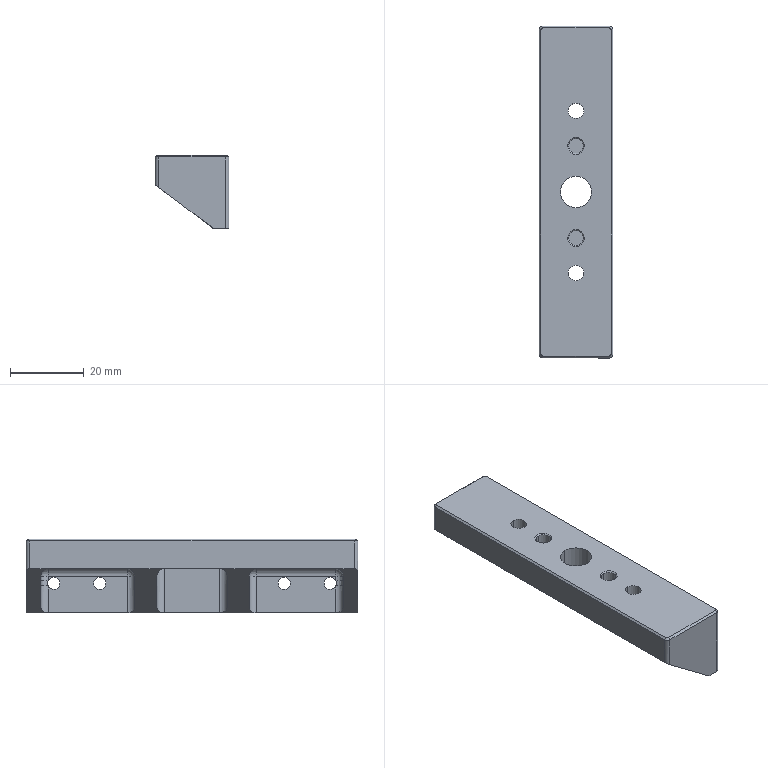NC program | NX | posted with a generic post | part box 20 x 90 x 20 mm
Whole program:
N10 G17 G21 G94 G90
(DRILLING_COPY , TOOL : D6A45)
N12 T01 M6
N14 G54
N16 G17 G0 G90 X-37.5 Y-2. B0. C0. S5000 M3
N18 G43 Z30. H1
N20 G94 G81 G98 Z-1. F350. R3.
N22 X-25.
N24 X-12.5
N26 X12.5
N28 X25.
N30 X37.5
N32 G80
N34 G0 X37.5 Y-2. Z30.
N36 M5
(DRILLING_COPY_1 , TOOL : 3.3ZT)
N38 T03 M6
N40 G54
N42 G17 G0 G90 X-37.5 Y-2. B0. C0. S2000 M3
N44 G43 Z30. H3
N46 G94 G83 G98 Z-6.491 F200. Q2. R3.
N48 X-25.
N50 X25.
N52 X37.5
N54 G80
N56 G0 X37.5 Y-2. Z30.
N58 M5
(DRILLING_COPY_COPY_1_COPY_COPY , TOOL : 3.8ZT)
N60 T18 M6
N62 G54
N64 G17 G0 G90 X12.5 Y-2. B0. C0. S2000 M3
N66 G43 Z30. H18
N68 G94 G83 G98 Z-5.142 F200. Q2. R3.
N70 X-12.5
N72 G80
N74 G0 X-12.5 Y-2. Z30.
N76 M5
(PLANAR_MILL_COPY_COPY_COPY_COPY_2 , TOOL : D6A45)
N78 T01 M6
N80 G54
N82 G17 G0 G90 X37.924 Y-2.626 B0. C0. S9500 M3
N84 G43 Z30. H1
N86 Z0.5
N88 G94 G1 X38.052 Y-2.552 Z0.46 F1250.
N90 X38.25 Y-2.214 Z0.356
N92 Y-1.786 Z0.241
N94 X38.052 Y-1.448 Z0.136
N96 X37.714 Y-1.25 Z0.031
N98 X37.286 Z-0.084
N100 X36.948 Y-1.448 Z-0.189
N102 X36.75 Y-1.786 Z-0.294
N104 Y-2.214 Z-0.408
N106 X36.948 Y-2.552 Z-0.513
N108 X37.286 Y-2.75 Z-0.618
N110 X37.714 Z-0.733
N112 X38.052 Y-2.552 Z-0.838
N114 X38.25 Y-2.214 Z-0.943
N116 Y-2. Z-1.
N118 G3 X37.5 Y-1.25 R0.75
N120 X38.25 Y-2. R-0.75
N122 X38. Y-1.567 R0.5
N124 G1 Z0.5
N126 G0 Z30.
N128 X24.374 Y-2.424
N130 Z0.5
N132 G1 X24.448 Y-2.552 Z0.46
N134 X24.786 Y-2.75 Z0.356
N136 X25.214 Z0.241
N138 X25.552 Y-2.552 Z0.136
N140 X25.75 Y-2.214 Z0.031
N142 Y-1.786 Z-0.084
N144 X25.552 Y-1.448 Z-0.189
N146 X25.214 Y-1.25 Z-0.294
N148 X24.786 Z-0.408
N150 X24.448 Y-1.448 Z-0.513
N152 X24.25 Y-1.786 Z-0.618
N154 Y-2.214 Z-0.733
N156 X24.448 Y-2.552 Z-0.838
N158 X24.786 Y-2.75 Z-0.943
N160 X25. Z-1.
N162 G3 X25.75 Y-2. R0.75
N164 X25. Y-2.75 R-0.75
N166 X25.433 Y-2.5 R0.5
N168 G1 Z0.5
N170 G0 Z30.
N172 X12.361 Y-2.144
N174 Z0.5
N176 G1 Z-1.
N178 X11.634 Y-2.9
N180 G3 X12.5 Y-3.4 R1.
N182 X13.9 Y-2. R1.4
N184 X12.5 Y-3.4 R-1.4
N186 X13.366 Y-2.9 R1.
N188 G1 X12.639 Y-2.144
N190 Z0.5
N192 G0 Z30.
N194 X-12.639
N196 Z0.5
N198 G1 Z-1.
N200 X-13.366 Y-2.9
N202 G3 X-12.5 Y-3.4 R1.
N204 X-11.1 Y-2. R1.4
N206 X-12.5 Y-3.4 R-1.4
N208 X-11.634 Y-2.9 R1.
N210 G1 X-12.361 Y-2.144
N212 Z0.5
N214 G0 Z30.
N216 X-25.626 Y-2.424
N218 Z0.5
N220 G1 X-25.552 Y-2.552 Z0.46
N222 X-25.214 Y-2.75 Z0.356
N224 X-24.786 Z0.241
N226 X-24.448 Y-2.552 Z0.136
N228 X-24.25 Y-2.214 Z0.031
N230 Y-1.786 Z-0.084
N232 X-24.448 Y-1.448 Z-0.189
N234 X-24.786 Y-1.25 Z-0.294
N236 X-25.214 Z-0.408
N238 X-25.552 Y-1.448 Z-0.513
N240 X-25.75 Y-1.786 Z-0.618
N242 Y-2.214 Z-0.733
N244 X-25.552 Y-2.552 Z-0.838
N246 X-25.214 Y-2.75 Z-0.943
N248 X-25. Z-1.
N250 G3 X-24.25 Y-2. R0.75
N252 X-25. Y-2.75 R-0.75
N254 X-24.567 Y-2.5 R0.5
N256 G1 Z0.5
N258 G0 Z30.
N260 X-37.924 Y-1.374
N262 Z0.5
N264 G1 X-38.052 Y-1.448 Z0.46
N266 X-38.25 Y-1.786 Z0.356
N268 Y-2.214 Z0.241
N270 X-38.052 Y-2.552 Z0.136
N272 X-37.714 Y-2.75 Z0.031
N274 X-37.286 Z-0.084
N276 X-36.948 Y-2.552 Z-0.189
N278 X-36.75 Y-2.214 Z-0.294
N280 Y-1.786 Z-0.408
N282 X-36.948 Y-1.448 Z-0.513
N284 X-37.286 Y-1.25 Z-0.618
N286 X-37.714 Z-0.733
N288 X-38.052 Y-1.448 Z-0.838
N290 X-38.25 Y-1.786 Z-0.943
N292 Y-2. Z-1.
N294 G3 X-37.5 Y-2.75 R0.75
N296 X-38.25 Y-2. R-0.75
N298 X-38. Y-2.433 R0.5
N300 G1 Z0.5
N302 G0 Z30.
N304 M5
(刀补_COPY , TOOL : D3)
N306 T17 M6
N308 G54
N310 G17 G0 G90 X-12.5 Y-2. B0. C0. S9500 M3
N312 G43 Z30. H17
N314 Z0.5
N316 G41 G94 G1 X-12.473 Y-2.096 F1250. D17
N318 G3 X-12.05 Y-2. R0.222
N320 X-12.05 Y-2. Z-0.5 I-0.45 J0.
N322 X-12.05 Y-2. Z-1.5 I-0.45 J0.
N324 X-12.05 Y-2. Z-2.5 I-0.45 J0.
N326 X-12.05 Y-2. Z-3.5 I-0.45 J0.
N328 X-12.95 Y-2. Z-4. I-0.45 J0.
N330 X-12.5 Y-2.45 R0.45
N332 X-12.95 Y-2. R-0.45
N334 X-12.527 Y-2.096 R0.222
N336 G40
N338 G1 X-12.5 Y-2.
N340 G0 Z30.
N342 X12.5
N344 Z0.5
N346 G41 G1 X12.527 Y-2.096
N348 G3 X12.95 Y-2. R0.222
N350 X12.95 Y-2. Z-0.5 I-0.45 J0.
N352 X12.95 Y-2. Z-1.5 I-0.45 J0.
N354 X12.95 Y-2. Z-2.5 I-0.45 J0.
N356 X12.95 Y-2. Z-3.5 I-0.45 J0.
N358 X12.05 Y-2. Z-4. I-0.45 J0.
N360 X12.5 Y-2.45 R0.45
N362 X12.05 Y-2. R-0.45
N364 X12.473 Y-2.096 R0.222
N366 G40
N368 G1 X12.5 Y-2.
N370 G0 Z30.
N372 M5
N374 M2